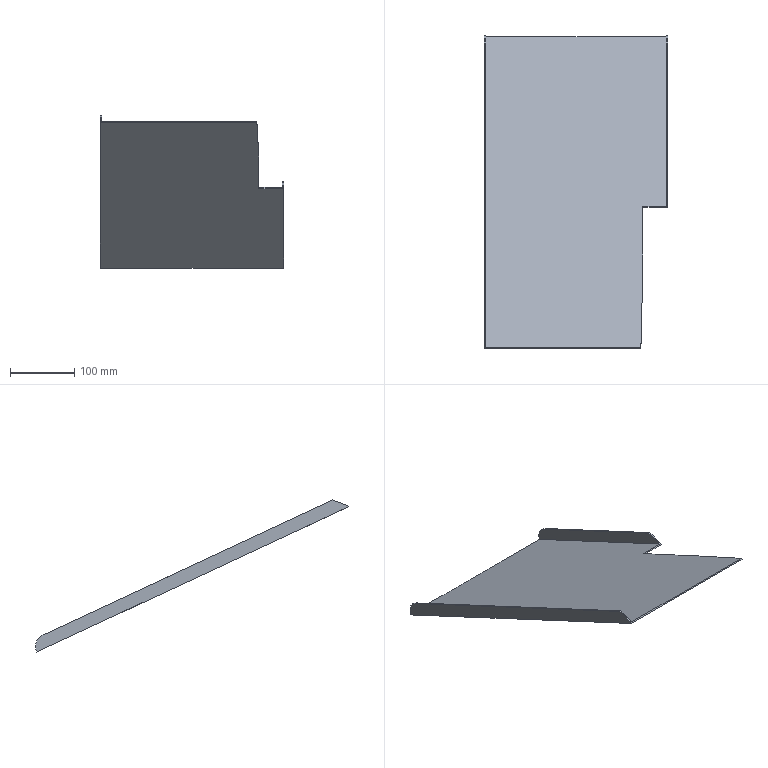Part | NX | features solid 2 | 1 solid | 17 faces | box 284.627 x 485.226 x 235.91 mm | volume 312843 mm3 | plane 14 | cylinder 2 | spline 1 | commonest cylinder face diameters 40 x2
STEP:
#1=CARTESIAN_POINT('',(-367.373,820.,-334.717));
#2=VERTEX_POINT('',#1);
#3=CARTESIAN_POINT('',(-367.373,820.,-332.51));
#4=VERTEX_POINT('',#3);
#5=CARTESIAN_POINT('',(-367.373,820.,-700.));
#6=DIRECTION('',(0.,0.,1.));
#7=VECTOR('',#6,1000.);
#8=LINE('',#5,#7);
#9=EDGE_CURVE('',#2,#4,#8,.T.);
#10=ORIENTED_EDGE('',*,*,#9,.F.);
#11=CARTESIAN_POINT('',(-648.,820.,-334.717));
#12=VERTEX_POINT('',#11);
#13=CARTESIAN_POINT('',(-419.852,820.,-334.717));
#14=DIRECTION('',(-1.,0.,0.));
#15=VECTOR('',#14,1000.);
#16=LINE('',#13,#15);
#17=EDGE_CURVE('',#2,#12,#16,.T.);
#18=ORIENTED_EDGE('',*,*,#17,.T.);
#19=CARTESIAN_POINT('',(-648.,820.,-332.51));
#20=VERTEX_POINT('',#19);
#21=CARTESIAN_POINT('',(-648.,820.,-700.));
#22=DIRECTION('',(0.,0.,-1.));
#23=VECTOR('',#22,1000.);
#24=LINE('',#21,#23);
#25=EDGE_CURVE('',#20,#12,#24,.T.);
#26=ORIENTED_EDGE('',*,*,#25,.F.);
#27=CARTESIAN_POINT('',(-419.852,820.,-332.51));
#28=DIRECTION('',(-1.,0.,0.));
#29=VECTOR('',#28,1000.);
#30=LINE('',#27,#29);
#31=EDGE_CURVE('',#4,#20,#30,.T.);
#32=ORIENTED_EDGE('',*,*,#31,.F.);
#33=EDGE_LOOP('',(#10,#18,#26,#32));
#34=FACE_BOUND('',#33,.T.);
#35=CARTESIAN_POINT('',(1065.,820.,-700.));
#36=DIRECTION('',(0.,-1.,0.));
#37=DIRECTION('',(-1.,0.,0.));
#38=AXIS2_PLACEMENT_3D('',#35,#36,#37);
#39=PLANE('',#38);
#40=ADVANCED_FACE('',(#34),#39,.F.);
#41=CARTESIAN_POINT('',(-367.373,556.481,-209.629));
#42=VERTEX_POINT('',#41);
#43=CARTESIAN_POINT('',(-367.373,317.493,-98.187));
#44=DIRECTION('',(0.,-0.9063,0.4226));
#45=VECTOR('',#44,1000.);
#46=LINE('',#43,#45);
#47=EDGE_CURVE('',#4,#42,#46,.T.);
#48=ORIENTED_EDGE('',*,*,#47,.F.);
#49=ORIENTED_EDGE('',*,*,#31,.T.);
#50=CARTESIAN_POINT('',(-648.,337.493,-107.514));
#51=VERTEX_POINT('',#50);
#52=CARTESIAN_POINT('',(-648.,317.493,-98.187));
#53=DIRECTION('',(0.,0.9063,-0.4226));
#54=VECTOR('',#53,1000.);
#55=LINE('',#52,#54);
#56=EDGE_CURVE('',#51,#20,#55,.T.);
#57=ORIENTED_EDGE('',*,*,#56,.F.);
#58=CARTESIAN_POINT('',(-407.057,337.493,-107.514));
#59=VERTEX_POINT('',#58);
#60=CARTESIAN_POINT('',(-419.852,337.493,-107.514));
#61=DIRECTION('',(-1.,0.,0.));
#62=VECTOR('',#61,1000.);
#63=LINE('',#60,#62);
#64=EDGE_CURVE('',#51,#59,#63,.F.);
#65=ORIENTED_EDGE('',*,*,#64,.T.);
#66=CARTESIAN_POINT('',(-404.001,556.494,-209.635));
#67=VERTEX_POINT('',#66);
#68=CARTESIAN_POINT('',(-407.057,337.493,-107.514));
#69=CARTESIAN_POINT('',(-406.902,341.01,-109.153));
#70=CARTESIAN_POINT('',(-406.6,348.566,-112.677));
#71=CARTESIAN_POINT('',(-406.245,359.315,-117.689));
#72=CARTESIAN_POINT('',(-405.973,368.697,-122.064));
#73=CARTESIAN_POINT('',(-405.808,374.888,-124.951));
#74=CARTESIAN_POINT('',(-405.68,380.035,-127.351));
#75=CARTESIAN_POINT('',(-405.585,383.996,-129.198));
#76=CARTESIAN_POINT('',(-405.507,387.368,-130.77));
#77=CARTESIAN_POINT('',(-405.453,389.792,-131.901));
#78=CARTESIAN_POINT('',(-405.423,391.156,-132.537));
#79=CARTESIAN_POINT('',(-405.399,392.28,-133.061));
#80=CARTESIAN_POINT('',(-405.382,393.048,-133.419));
#81=CARTESIAN_POINT('',(-405.358,394.196,-133.954));
#82=CARTESIAN_POINT('',(-405.316,396.148,-134.865));
#83=CARTESIAN_POINT('',(-405.258,398.972,-136.182));
#84=CARTESIAN_POINT('',(-405.19,402.355,-137.759));
#85=CARTESIAN_POINT('',(-405.102,406.878,-139.868));
#86=CARTESIAN_POINT('',(-404.997,412.548,-142.512));
#87=CARTESIAN_POINT('',(-404.84,421.657,-146.76));
#88=CARTESIAN_POINT('',(-404.699,430.812,-151.029));
#89=CARTESIAN_POINT('',(-404.589,438.887,-154.794));
#90=CARTESIAN_POINT('',(-404.531,443.489,-156.94));
#91=CARTESIAN_POINT('',(-404.488,447.022,-158.587));
#92=CARTESIAN_POINT('',(-404.45,450.273,-160.103));
#93=CARTESIAN_POINT('',(-404.401,454.73,-162.182));
#94=CARTESIAN_POINT('',(-404.322,462.533,-165.821));
#95=CARTESIAN_POINT('',(-404.245,471.588,-170.043));
#96=CARTESIAN_POINT('',(-404.181,480.752,-174.316));
#97=CARTESIAN_POINT('',(-404.147,486.53,-177.01));
#98=CARTESIAN_POINT('',(-404.123,491.18,-179.179));
#99=CARTESIAN_POINT('',(-404.107,494.685,-180.813));
#100=CARTESIAN_POINT('',(-404.095,497.607,-182.176));
#101=CARTESIAN_POINT('',(-404.087,499.681,-183.143));
#102=CARTESIAN_POINT('',(-404.083,500.833,-183.68));
#103=CARTESIAN_POINT('',(-404.079,501.795,-184.129));
#104=CARTESIAN_POINT('',(-404.078,502.388,-184.405));
#105=CARTESIAN_POINT('',(-404.074,503.324,-184.842));
#106=CARTESIAN_POINT('',(-404.069,504.937,-185.594));
#107=CARTESIAN_POINT('',(-404.063,507.377,-186.732));
#108=CARTESIAN_POINT('',(-404.055,510.455,-188.167));
#109=CARTESIAN_POINT('',(-404.046,514.785,-190.186));
#110=CARTESIAN_POINT('',(-404.037,519.44,-192.357));
#111=CARTESIAN_POINT('',(-404.031,524.43,-194.684));
#112=CARTESIAN_POINT('',(-404.027,527.677,-196.198));
#113=CARTESIAN_POINT('',(-404.024,530.378,-197.457));
#114=CARTESIAN_POINT('',(-404.022,531.884,-198.159));
#115=CARTESIAN_POINT('',(-404.021,532.972,-198.667));
#116=CARTESIAN_POINT('',(-404.021,533.53,-198.927));
#117=CARTESIAN_POINT('',(-404.02,534.536,-199.396));
#118=CARTESIAN_POINT('',(-404.018,536.527,-200.325));
#119=CARTESIAN_POINT('',(-404.016,539.382,-201.656));
#120=CARTESIAN_POINT('',(-404.012,543.944,-203.783));
#121=CARTESIAN_POINT('',(-404.007,549.649,-206.444));
#122=CARTESIAN_POINT('',(-404.003,554.212,-208.571));
#123=CARTESIAN_POINT('',(-404.001,556.494,-209.635));
#124=B_SPLINE_CURVE_WITH_KNOTS('',3,(#68,#69,#70,#71,#72,#73,#74,#75,#76,#77,#78,#79,#80,#81,#82,#83,#84,#85,#86,#87,#88,#89,#90,#91,#92,#93,#94,#95,#96,#97,#98,#99,#100,#101,#102,#103,#104,#105,#106,#107,#108,#109,#110,#111,#112,#113,#114,#115,#116,#117,#118,#119,#120,#121,#122,#123),.UNSPECIFIED.,.F.,.F.,(4,1,1,1,1,1,1,1,1,1,1,1,1,1,1,1,1,1,1,1,1,1,1,1,1,1,1,1,1,1,1,1,1,1,1,1,1,1,1,1,1,1,1,1,1,1,1,1,1,1,1,1,1,4),(0.,0.0625,0.125,0.1562,0.1875,0.2031,0.2188,0.2344,0.2422,0.2461,0.25,0.2539,0.2578,0.2656,0.2812,0.2969,0.3125,0.3438,0.375,0.4375,0.4688,0.4844,0.5,0.5156,0.5312,0.5625,0.625,0.6562,0.6875,0.7031,0.7188,0.7344,0.7422,0.7461,0.75,0.7539,0.7578,0.7656,0.7812,0.7969,0.8125,0.8438,0.8594,0.875,0.8828,0.8906,0.8926,0.8945,0.8984,0.9062,0.9219,0.9375,0.9688,1.),.UNSPECIFIED.);
#125=EDGE_CURVE('',#67,#59,#124,.F.);
#126=ORIENTED_EDGE('',*,*,#125,.F.);
#127=CARTESIAN_POINT('',(-404.001,556.494,-209.635));
#128=CARTESIAN_POINT('',(-391.792,556.49,-209.633));
#129=CARTESIAN_POINT('',(-379.582,556.485,-209.631));
#130=CARTESIAN_POINT('',(-367.373,556.481,-209.629));
#131=B_SPLINE_CURVE_WITH_KNOTS('',3,(#127,#128,#129,#130),.UNSPECIFIED.,.F.,.F.,(4,4),(0.,0.9482),.UNSPECIFIED.);
#132=EDGE_CURVE('',#67,#42,#131,.T.);
#133=ORIENTED_EDGE('',*,*,#132,.T.);
#134=EDGE_LOOP('',(#48,#49,#57,#65,#126,#133));
#135=FACE_BOUND('',#134,.T.);
#136=CARTESIAN_POINT('',(-419.852,317.493,-98.187));
#137=DIRECTION('',(0.,-0.4226,-0.9063));
#138=DIRECTION('',(-1.,0.,0.));
#139=AXIS2_PLACEMENT_3D('',#136,#137,#138);
#140=PLANE('',#139);
#141=ADVANCED_FACE('',(#135),#140,.F.);
#142=CARTESIAN_POINT('',(-367.373,555.635,-211.442));
#143=VERTEX_POINT('',#142);
#144=CARTESIAN_POINT('',(-367.373,556.481,-209.629));
#145=CARTESIAN_POINT('',(-367.373,556.199,-210.234));
#146=CARTESIAN_POINT('',(-367.373,555.917,-210.838));
#147=CARTESIAN_POINT('',(-367.373,555.635,-211.443));
#148=B_SPLINE_CURVE_WITH_KNOTS('',3,(#144,#145,#146,#147),.UNSPECIFIED.,.F.,.F.,(4,4),(0.,1.),.UNSPECIFIED.);
#149=EDGE_CURVE('',#143,#42,#148,.F.);
#150=ORIENTED_EDGE('',*,*,#149,.T.);
#151=ORIENTED_EDGE('',*,*,#132,.F.);
#152=CARTESIAN_POINT('',(-404.001,555.649,-211.448));
#153=VERTEX_POINT('',#152);
#154=CARTESIAN_POINT('',(-404.001,556.494,-209.635));
#155=CARTESIAN_POINT('',(-404.001,556.212,-210.24));
#156=CARTESIAN_POINT('',(-404.001,555.931,-210.844));
#157=CARTESIAN_POINT('',(-404.001,555.649,-211.448));
#158=B_SPLINE_CURVE_WITH_KNOTS('',3,(#154,#155,#156,#157),.UNSPECIFIED.,.F.,.F.,(4,4),(0.,1.),.UNSPECIFIED.);
#159=EDGE_CURVE('',#67,#153,#158,.T.);
#160=ORIENTED_EDGE('',*,*,#159,.T.);
#161=CARTESIAN_POINT('',(-404.001,555.649,-211.448));
#162=CARTESIAN_POINT('',(-391.792,555.644,-211.446));
#163=CARTESIAN_POINT('',(-379.582,555.64,-211.444));
#164=CARTESIAN_POINT('',(-367.373,555.635,-211.442));
#165=B_SPLINE_CURVE_WITH_KNOTS('',3,(#161,#162,#163,#164),.UNSPECIFIED.,.F.,.F.,(4,4),(0.,0.9482),.UNSPECIFIED.);
#166=EDGE_CURVE('',#153,#143,#165,.T.);
#167=ORIENTED_EDGE('',*,*,#166,.T.);
#168=EDGE_LOOP('',(#150,#151,#160,#167));
#169=FACE_BOUND('',#168,.T.);
#170=CARTESIAN_POINT('',(-404.001,556.494,-209.635));
#171=DIRECTION('',(0.0004088,0.9063,-0.4226));
#172=DIRECTION('',(0.,0.4226,0.9063));
#173=AXIS2_PLACEMENT_3D('',#170,#171,#172);
#174=PLANE('',#173);
#175=ADVANCED_FACE('',(#169),#174,.F.);
#176=CARTESIAN_POINT('',(-365.373,555.635,-211.441));
#177=VERTEX_POINT('',#176);
#178=CARTESIAN_POINT('',(-365.373,820.,-334.717));
#179=VERTEX_POINT('',#178);
#180=CARTESIAN_POINT('',(-365.373,543.591,-205.825));
#181=DIRECTION('',(0.,-0.9063,0.4226));
#182=VECTOR('',#181,1000.);
#183=LINE('',#180,#182);
#184=EDGE_CURVE('',#177,#179,#183,.F.);
#185=ORIENTED_EDGE('',*,*,#184,.T.);
#186=CARTESIAN_POINT('',(-365.373,810.326,-308.138));
#187=VERTEX_POINT('',#186);
#188=CARTESIAN_POINT('',(-365.373,801.874,-326.265));
#189=DIRECTION('',(1.,0.,0.));
#190=DIRECTION('',(0.,1.,0.));
#191=AXIS2_PLACEMENT_3D('',#188,#189,#190);
#192=CIRCLE('',#191,20.);
#193=EDGE_CURVE('',#179,#187,#192,.T.);
#194=ORIENTED_EDGE('',*,*,#193,.T.);
#195=CARTESIAN_POINT('',(-365.373,580.401,-200.922));
#196=VERTEX_POINT('',#195);
#197=CARTESIAN_POINT('',(-365.373,564.087,-193.315));
#198=DIRECTION('',(0.,0.9063,-0.4226));
#199=VECTOR('',#198,1000.);
#200=LINE('',#197,#199);
#201=EDGE_CURVE('',#196,#187,#200,.T.);
#202=ORIENTED_EDGE('',*,*,#201,.F.);
#203=CARTESIAN_POINT('',(-365.373,556.48,-209.629));
#204=VERTEX_POINT('',#203);
#205=CARTESIAN_POINT('',(-365.373,555.151,-210.112));
#206=DIRECTION('',(0.,0.9397,0.342));
#207=VECTOR('',#206,1000.);
#208=LINE('',#205,#207);
#209=EDGE_CURVE('',#196,#204,#208,.F.);
#210=ORIENTED_EDGE('',*,*,#209,.T.);
#211=CARTESIAN_POINT('',(-365.373,556.48,-209.629));
#212=CARTESIAN_POINT('',(-365.373,556.198,-210.233));
#213=CARTESIAN_POINT('',(-365.373,555.916,-210.837));
#214=CARTESIAN_POINT('',(-365.373,555.635,-211.441));
#215=B_SPLINE_CURVE_WITH_KNOTS('',3,(#211,#212,#213,#214),.UNSPECIFIED.,.F.,.F.,(4,4),(0.,1.),.UNSPECIFIED.);
#216=EDGE_CURVE('',#177,#204,#215,.F.);
#217=ORIENTED_EDGE('',*,*,#216,.F.);
#218=EDGE_LOOP('',(#185,#194,#202,#210,#217));
#219=FACE_BOUND('',#218,.T.);
#220=CARTESIAN_POINT('',(-365.373,544.437,-204.013));
#221=DIRECTION('',(-1.,0.,0.));
#222=DIRECTION('',(0.,-1.,0.));
#223=AXIS2_PLACEMENT_3D('',#220,#221,#222);
#224=PLANE('',#223);
#225=ADVANCED_FACE('',(#219),#224,.F.);
#226=CARTESIAN_POINT('',(-650.,810.326,-308.138));
#227=VERTEX_POINT('',#226);
#228=CARTESIAN_POINT('',(-650.,820.,-334.717));
#229=VERTEX_POINT('',#228);
#230=CARTESIAN_POINT('',(-650.,801.874,-326.265));
#231=DIRECTION('',(-1.,0.,0.));
#232=DIRECTION('',(0.,0.,1.));
#233=AXIS2_PLACEMENT_3D('',#230,#231,#232);
#234=CIRCLE('',#233,20.);
#235=EDGE_CURVE('',#227,#229,#234,.T.);
#236=ORIENTED_EDGE('',*,*,#235,.T.);
#237=CARTESIAN_POINT('',(-650.,336.648,-109.326));
#238=VERTEX_POINT('',#237);
#239=CARTESIAN_POINT('',(-650.,-1117.742,568.867));
#240=DIRECTION('',(0.,-0.9063,0.4226));
#241=VECTOR('',#240,1000.);
#242=LINE('',#239,#241);
#243=EDGE_CURVE('',#229,#238,#242,.T.);
#244=ORIENTED_EDGE('',*,*,#243,.T.);
#245=CARTESIAN_POINT('',(-650.,337.493,-107.514));
#246=VERTEX_POINT('',#245);
#247=CARTESIAN_POINT('',(-650.,337.493,-107.514));
#248=DIRECTION('',(0.,-0.4226,-0.9063));
#249=VECTOR('',#248,1000.);
#250=LINE('',#247,#249);
#251=EDGE_CURVE('',#246,#238,#250,.T.);
#252=ORIENTED_EDGE('',*,*,#251,.F.);
#253=CARTESIAN_POINT('',(-650.,361.414,-98.807));
#254=VERTEX_POINT('',#253);
#255=CARTESIAN_POINT('',(-650.,690.536,20.983));
#256=DIRECTION('',(0.,0.9397,0.342));
#257=VECTOR('',#256,1000.);
#258=LINE('',#255,#257);
#259=EDGE_CURVE('',#246,#254,#258,.T.);
#260=ORIENTED_EDGE('',*,*,#259,.T.);
#261=CARTESIAN_POINT('',(-650.,828.452,-316.591));
#262=DIRECTION('',(0.,-0.9063,0.4226));
#263=VECTOR('',#262,1000.);
#264=LINE('',#261,#263);
#265=EDGE_CURVE('',#227,#254,#264,.T.);
#266=ORIENTED_EDGE('',*,*,#265,.F.);
#267=EDGE_LOOP('',(#236,#244,#252,#260,#266));
#268=FACE_BOUND('',#267,.T.);
#269=CARTESIAN_POINT('',(-650.,-1116.896,570.679));
#270=DIRECTION('',(1.,0.,0.));
#271=DIRECTION('',(0.,0.,-1.));
#272=AXIS2_PLACEMENT_3D('',#269,#270,#271);
#273=PLANE('',#272);
#274=ADVANCED_FACE('',(#268),#273,.F.);
#275=CARTESIAN_POINT('',(-407.057,336.648,-109.326));
#276=VERTEX_POINT('',#275);
#277=CARTESIAN_POINT('',(-419.852,336.648,-109.326));
#278=DIRECTION('',(-1.,0.,0.));
#279=VECTOR('',#278,1000.);
#280=LINE('',#277,#279);
#281=EDGE_CURVE('',#238,#276,#280,.F.);
#282=ORIENTED_EDGE('',*,*,#281,.T.);
#283=CARTESIAN_POINT('',(-407.057,336.648,-109.326));
#284=CARTESIAN_POINT('',(-407.057,336.93,-108.722));
#285=CARTESIAN_POINT('',(-407.057,337.212,-108.118));
#286=CARTESIAN_POINT('',(-407.057,337.493,-107.514));
#287=B_SPLINE_CURVE_WITH_KNOTS('',3,(#283,#284,#285,#286),.UNSPECIFIED.,.F.,.F.,(4,4),(0.,1.),.UNSPECIFIED.);
#288=EDGE_CURVE('',#59,#276,#287,.F.);
#289=ORIENTED_EDGE('',*,*,#288,.F.);
#290=ORIENTED_EDGE('',*,*,#64,.F.);
#291=CARTESIAN_POINT('',(-419.852,337.493,-107.514));
#292=DIRECTION('',(-1.,0.,0.));
#293=VECTOR('',#292,1000.);
#294=LINE('',#291,#293);
#295=EDGE_CURVE('',#246,#51,#294,.F.);
#296=ORIENTED_EDGE('',*,*,#295,.F.);
#297=ORIENTED_EDGE('',*,*,#251,.T.);
#298=EDGE_LOOP('',(#282,#289,#290,#296,#297));
#299=FACE_BOUND('',#298,.T.);
#300=CARTESIAN_POINT('',(-419.852,337.493,-107.514));
#301=DIRECTION('',(0.,0.9063,-0.4226));
#302=DIRECTION('',(0.,0.4226,0.9063));
#303=AXIS2_PLACEMENT_3D('',#300,#301,#302);
#304=PLANE('',#303);
#305=ADVANCED_FACE('',(#299),#304,.F.);
#306=CARTESIAN_POINT('',(-407.057,336.648,-109.326));
#307=CARTESIAN_POINT('',(-406.902,340.165,-110.966));
#308=CARTESIAN_POINT('',(-406.6,347.721,-114.489));
#309=CARTESIAN_POINT('',(-406.245,358.47,-119.502));
#310=CARTESIAN_POINT('',(-405.973,367.852,-123.877));
#311=CARTESIAN_POINT('',(-405.808,374.042,-126.763));
#312=CARTESIAN_POINT('',(-405.68,379.189,-129.163));
#313=CARTESIAN_POINT('',(-405.585,383.151,-131.011));
#314=CARTESIAN_POINT('',(-405.507,386.522,-132.583));
#315=CARTESIAN_POINT('',(-405.453,388.947,-133.714));
#316=CARTESIAN_POINT('',(-405.423,390.311,-134.35));
#317=CARTESIAN_POINT('',(-405.399,391.435,-134.874));
#318=CARTESIAN_POINT('',(-405.382,392.202,-135.232));
#319=CARTESIAN_POINT('',(-405.358,393.351,-135.767));
#320=CARTESIAN_POINT('',(-405.316,395.303,-136.677));
#321=CARTESIAN_POINT('',(-405.258,398.127,-137.994));
#322=CARTESIAN_POINT('',(-405.19,401.51,-139.572));
#323=CARTESIAN_POINT('',(-405.102,406.033,-141.681));
#324=CARTESIAN_POINT('',(-404.997,411.703,-144.325));
#325=CARTESIAN_POINT('',(-404.84,420.811,-148.572));
#326=CARTESIAN_POINT('',(-404.699,429.967,-152.841));
#327=CARTESIAN_POINT('',(-404.589,438.042,-156.607));
#328=CARTESIAN_POINT('',(-404.531,442.643,-158.753));
#329=CARTESIAN_POINT('',(-404.488,446.176,-160.4));
#330=CARTESIAN_POINT('',(-404.45,449.427,-161.916));
#331=CARTESIAN_POINT('',(-404.401,453.885,-163.995));
#332=CARTESIAN_POINT('',(-404.322,461.688,-167.633));
#333=CARTESIAN_POINT('',(-404.245,470.743,-171.856));
#334=CARTESIAN_POINT('',(-404.181,479.907,-176.129));
#335=CARTESIAN_POINT('',(-404.147,485.685,-178.823));
#336=CARTESIAN_POINT('',(-404.123,490.334,-180.991));
#337=CARTESIAN_POINT('',(-404.107,493.84,-182.626));
#338=CARTESIAN_POINT('',(-404.095,496.762,-183.988));
#339=CARTESIAN_POINT('',(-404.087,498.835,-184.955));
#340=CARTESIAN_POINT('',(-404.083,499.988,-185.493));
#341=CARTESIAN_POINT('',(-404.079,500.95,-185.941));
#342=CARTESIAN_POINT('',(-404.078,501.543,-186.218));
#343=CARTESIAN_POINT('',(-404.074,502.479,-186.654));
#344=CARTESIAN_POINT('',(-404.069,504.092,-187.407));
#345=CARTESIAN_POINT('',(-404.063,506.532,-188.544));
#346=CARTESIAN_POINT('',(-404.055,509.61,-189.98));
#347=CARTESIAN_POINT('',(-404.046,513.939,-191.998));
#348=CARTESIAN_POINT('',(-404.037,518.595,-194.169));
#349=CARTESIAN_POINT('',(-404.031,523.585,-196.496));
#350=CARTESIAN_POINT('',(-404.027,526.832,-198.01));
#351=CARTESIAN_POINT('',(-404.024,529.533,-199.27));
#352=CARTESIAN_POINT('',(-404.022,531.039,-199.972));
#353=CARTESIAN_POINT('',(-404.021,532.126,-200.479));
#354=CARTESIAN_POINT('',(-404.021,532.685,-200.74));
#355=CARTESIAN_POINT('',(-404.02,533.691,-201.209));
#356=CARTESIAN_POINT('',(-404.018,535.682,-202.137));
#357=CARTESIAN_POINT('',(-404.016,538.537,-203.469));
#358=CARTESIAN_POINT('',(-404.012,543.099,-205.596));
#359=CARTESIAN_POINT('',(-404.007,548.804,-208.256));
#360=CARTESIAN_POINT('',(-404.003,553.367,-210.384));
#361=CARTESIAN_POINT('',(-404.001,555.649,-211.448));
#362=B_SPLINE_CURVE_WITH_KNOTS('',3,(#306,#307,#308,#309,#310,#311,#312,#313,#314,#315,#316,#317,#318,#319,#320,#321,#322,#323,#324,#325,#326,#327,#328,#329,#330,#331,#332,#333,#334,#335,#336,#337,#338,#339,#340,#341,#342,#343,#344,#345,#346,#347,#348,#349,#350,#351,#352,#353,#354,#355,#356,#357,#358,#359,#360,#361),.UNSPECIFIED.,.F.,.F.,(4,1,1,1,1,1,1,1,1,1,1,1,1,1,1,1,1,1,1,1,1,1,1,1,1,1,1,1,1,1,1,1,1,1,1,1,1,1,1,1,1,1,1,1,1,1,1,1,1,1,1,1,1,4),(0.,0.0625,0.125,0.1562,0.1875,0.2031,0.2188,0.2344,0.2422,0.2461,0.25,0.2539,0.2578,0.2656,0.2812,0.2969,0.3125,0.3438,0.375,0.4375,0.4688,0.4844,0.5,0.5156,0.5312,0.5625,0.625,0.6562,0.6875,0.7031,0.7188,0.7344,0.7422,0.7461,0.75,0.7539,0.7578,0.7656,0.7812,0.7969,0.8125,0.8438,0.8594,0.875,0.8828,0.8906,0.8926,0.8945,0.8984,0.9062,0.9219,0.9375,0.9688,1.),.UNSPECIFIED.);
#363=EDGE_CURVE('',#153,#276,#362,.F.);
#364=ORIENTED_EDGE('',*,*,#363,.F.);
#365=ORIENTED_EDGE('',*,*,#159,.F.);
#366=ORIENTED_EDGE('',*,*,#125,.T.);
#367=ORIENTED_EDGE('',*,*,#288,.T.);
#368=EDGE_LOOP('',(#364,#365,#366,#367));
#369=FACE_BOUND('',#368,.T.);
#370=CARTESIAN_POINT('',(-407.057,337.493,-107.514));
#371=CARTESIAN_POINT('',(-407.057,336.648,-109.326));
#372=CARTESIAN_POINT('',(-406.902,341.01,-109.153));
#373=CARTESIAN_POINT('',(-406.902,340.165,-110.966));
#374=CARTESIAN_POINT('',(-406.6,348.566,-112.677));
#375=CARTESIAN_POINT('',(-406.6,347.721,-114.489));
#376=CARTESIAN_POINT('',(-406.245,359.315,-117.689));
#377=CARTESIAN_POINT('',(-406.245,358.47,-119.502));
#378=CARTESIAN_POINT('',(-405.973,368.697,-122.064));
#379=CARTESIAN_POINT('',(-405.973,367.852,-123.877));
#380=CARTESIAN_POINT('',(-405.808,374.888,-124.951));
#381=CARTESIAN_POINT('',(-405.808,374.042,-126.763));
#382=CARTESIAN_POINT('',(-405.68,380.035,-127.351));
#383=CARTESIAN_POINT('',(-405.68,379.189,-129.163));
#384=CARTESIAN_POINT('',(-405.585,383.996,-129.198));
#385=CARTESIAN_POINT('',(-405.585,383.151,-131.011));
#386=CARTESIAN_POINT('',(-405.507,387.368,-130.77));
#387=CARTESIAN_POINT('',(-405.507,386.522,-132.583));
#388=CARTESIAN_POINT('',(-405.453,389.792,-131.901));
#389=CARTESIAN_POINT('',(-405.453,388.947,-133.714));
#390=CARTESIAN_POINT('',(-405.423,391.156,-132.537));
#391=CARTESIAN_POINT('',(-405.423,390.311,-134.35));
#392=CARTESIAN_POINT('',(-405.399,392.28,-133.061));
#393=CARTESIAN_POINT('',(-405.399,391.435,-134.874));
#394=CARTESIAN_POINT('',(-405.382,393.048,-133.419));
#395=CARTESIAN_POINT('',(-405.382,392.202,-135.232));
#396=CARTESIAN_POINT('',(-405.358,394.196,-133.954));
#397=CARTESIAN_POINT('',(-405.358,393.351,-135.767));
#398=CARTESIAN_POINT('',(-405.316,396.148,-134.865));
#399=CARTESIAN_POINT('',(-405.316,395.303,-136.677));
#400=CARTESIAN_POINT('',(-405.258,398.972,-136.182));
#401=CARTESIAN_POINT('',(-405.258,398.127,-137.994));
#402=CARTESIAN_POINT('',(-405.19,402.355,-137.759));
#403=CARTESIAN_POINT('',(-405.19,401.51,-139.572));
#404=CARTESIAN_POINT('',(-405.102,406.878,-139.868));
#405=CARTESIAN_POINT('',(-405.102,406.033,-141.681));
#406=CARTESIAN_POINT('',(-404.997,412.548,-142.512));
#407=CARTESIAN_POINT('',(-404.997,411.703,-144.325));
#408=CARTESIAN_POINT('',(-404.84,421.657,-146.76));
#409=CARTESIAN_POINT('',(-404.84,420.811,-148.572));
#410=CARTESIAN_POINT('',(-404.699,430.812,-151.029));
#411=CARTESIAN_POINT('',(-404.699,429.967,-152.841));
#412=CARTESIAN_POINT('',(-404.589,438.887,-154.794));
#413=CARTESIAN_POINT('',(-404.589,438.042,-156.607));
#414=CARTESIAN_POINT('',(-404.531,443.489,-156.94));
#415=CARTESIAN_POINT('',(-404.531,442.643,-158.753));
#416=CARTESIAN_POINT('',(-404.488,447.022,-158.587));
#417=CARTESIAN_POINT('',(-404.488,446.176,-160.4));
#418=CARTESIAN_POINT('',(-404.45,450.273,-160.103));
#419=CARTESIAN_POINT('',(-404.45,449.427,-161.916));
#420=CARTESIAN_POINT('',(-404.401,454.73,-162.182));
#421=CARTESIAN_POINT('',(-404.401,453.885,-163.995));
#422=CARTESIAN_POINT('',(-404.322,462.533,-165.821));
#423=CARTESIAN_POINT('',(-404.322,461.688,-167.633));
#424=CARTESIAN_POINT('',(-404.245,471.588,-170.043));
#425=CARTESIAN_POINT('',(-404.245,470.743,-171.856));
#426=CARTESIAN_POINT('',(-404.181,480.752,-174.316));
#427=CARTESIAN_POINT('',(-404.181,479.907,-176.129));
#428=CARTESIAN_POINT('',(-404.147,486.53,-177.01));
#429=CARTESIAN_POINT('',(-404.147,485.685,-178.823));
#430=CARTESIAN_POINT('',(-404.123,491.18,-179.179));
#431=CARTESIAN_POINT('',(-404.123,490.334,-180.991));
#432=CARTESIAN_POINT('',(-404.107,494.685,-180.813));
#433=CARTESIAN_POINT('',(-404.107,493.84,-182.626));
#434=CARTESIAN_POINT('',(-404.095,497.607,-182.176));
#435=CARTESIAN_POINT('',(-404.095,496.762,-183.988));
#436=CARTESIAN_POINT('',(-404.087,499.681,-183.143));
#437=CARTESIAN_POINT('',(-404.087,498.835,-184.955));
#438=CARTESIAN_POINT('',(-404.083,500.833,-183.68));
#439=CARTESIAN_POINT('',(-404.083,499.988,-185.493));
#440=CARTESIAN_POINT('',(-404.079,501.795,-184.129));
#441=CARTESIAN_POINT('',(-404.079,500.95,-185.941));
#442=CARTESIAN_POINT('',(-404.078,502.388,-184.405));
#443=CARTESIAN_POINT('',(-404.078,501.543,-186.218));
#444=CARTESIAN_POINT('',(-404.074,503.324,-184.842));
#445=CARTESIAN_POINT('',(-404.074,502.479,-186.654));
#446=CARTESIAN_POINT('',(-404.069,504.937,-185.594));
#447=CARTESIAN_POINT('',(-404.069,504.092,-187.407));
#448=CARTESIAN_POINT('',(-404.063,507.377,-186.732));
#449=CARTESIAN_POINT('',(-404.063,506.532,-188.544));
#450=CARTESIAN_POINT('',(-404.055,510.455,-188.167));
#451=CARTESIAN_POINT('',(-404.055,509.61,-189.98));
#452=CARTESIAN_POINT('',(-404.046,514.785,-190.186));
#453=CARTESIAN_POINT('',(-404.046,513.939,-191.998));
#454=CARTESIAN_POINT('',(-404.037,519.44,-192.357));
#455=CARTESIAN_POINT('',(-404.037,518.595,-194.169));
#456=CARTESIAN_POINT('',(-404.031,524.43,-194.684));
#457=CARTESIAN_POINT('',(-404.031,523.585,-196.496));
#458=CARTESIAN_POINT('',(-404.027,527.677,-196.198));
#459=CARTESIAN_POINT('',(-404.027,526.832,-198.01));
#460=CARTESIAN_POINT('',(-404.024,530.378,-197.457));
#461=CARTESIAN_POINT('',(-404.024,529.533,-199.27));
#462=CARTESIAN_POINT('',(-404.022,531.884,-198.159));
#463=CARTESIAN_POINT('',(-404.022,531.039,-199.972));
#464=CARTESIAN_POINT('',(-404.021,532.972,-198.667));
#465=CARTESIAN_POINT('',(-404.021,532.126,-200.479));
#466=CARTESIAN_POINT('',(-404.021,533.53,-198.927));
#467=CARTESIAN_POINT('',(-404.021,532.685,-200.74));
#468=CARTESIAN_POINT('',(-404.02,534.536,-199.396));
#469=CARTESIAN_POINT('',(-404.02,533.691,-201.209));
#470=CARTESIAN_POINT('',(-404.018,536.527,-200.325));
#471=CARTESIAN_POINT('',(-404.018,535.682,-202.137));
#472=CARTESIAN_POINT('',(-404.016,539.382,-201.656));
#473=CARTESIAN_POINT('',(-404.016,538.537,-203.469));
#474=CARTESIAN_POINT('',(-404.012,543.944,-203.783));
#475=CARTESIAN_POINT('',(-404.012,543.099,-205.596));
#476=CARTESIAN_POINT('',(-404.007,549.649,-206.444));
#477=CARTESIAN_POINT('',(-404.007,548.804,-208.256));
#478=CARTESIAN_POINT('',(-404.003,554.212,-208.571));
#479=CARTESIAN_POINT('',(-404.003,553.367,-210.384));
#480=CARTESIAN_POINT('',(-404.001,556.494,-209.635));
#481=CARTESIAN_POINT('',(-404.001,555.649,-211.448));
#482=B_SPLINE_SURFACE_WITH_KNOTS('',3,1,((#370,#371),(#372,#373),(#374,#375),(#376,#377),(#378,#379),(#380,#381),(#382,#383),(#384,#385),(#386,#387),(#388,#389),(#390,#391),(#392,#393),(#394,#395),(#396,#397),(#398,#399),(#400,#401),(#402,#403),(#404,#405),(#406,#407),(#408,#409),(#410,#411),(#412,#413),(#414,#415),(#416,#417),(#418,#419),(#420,#421),(#422,#423),(#424,#425),(#426,#427),(#428,#429),(#430,#431),(#432,#433),(#434,#435),(#436,#437),(#438,#439),(#440,#441),(#442,#443),(#444,#445),(#446,#447),(#448,#449),(#450,#451),(#452,#453),(#454,#455),(#456,#457),(#458,#459),(#460,#461),(#462,#463),(#464,#465),(#466,#467),(#468,#469),(#470,#471),(#472,#473),(#474,#475),(#476,#477),(#478,#479),(#480,#481)),.SURF_OF_LINEAR_EXTRUSION.,.F.,.F.,.F.,(4,1,1,1,1,1,1,1,1,1,1,1,1,1,1,1,1,1,1,1,1,1,1,1,1,1,1,1,1,1,1,1,1,1,1,1,1,1,1,1,1,1,1,1,1,1,1,1,1,1,1,1,1,4),(2,2),(0.,0.0625,0.125,0.1562,0.1875,0.2031,0.2188,0.2344,0.2422,0.2461,0.25,0.2539,0.2578,0.2656,0.2812,0.2969,0.3125,0.3438,0.375,0.4375,0.4688,0.4844,0.5,0.5156,0.5312,0.5625,0.625,0.6562,0.6875,0.7031,0.7188,0.7344,0.7422,0.7461,0.75,0.7539,0.7578,0.7656,0.7812,0.7969,0.8125,0.8438,0.8594,0.875,0.8828,0.8906,0.8926,0.8945,0.8984,0.9062,0.9219,0.9375,0.9688,1.),(0.,1.),.UNSPECIFIED.);
#483=ADVANCED_FACE('',(#369),#482,.F.);
#484=CARTESIAN_POINT('',(-367.373,555.635,-211.442));
#485=CARTESIAN_POINT('',(-366.706,555.635,-211.442));
#486=CARTESIAN_POINT('',(-366.039,555.635,-211.441));
#487=CARTESIAN_POINT('',(-365.373,555.635,-211.441));
#488=B_SPLINE_CURVE_WITH_KNOTS('',3,(#484,#485,#486,#487),.UNSPECIFIED.,.F.,.F.,(4,4),(0.9482,1.),.UNSPECIFIED.);
#489=EDGE_CURVE('',#177,#143,#488,.F.);
#490=ORIENTED_EDGE('',*,*,#489,.T.);
#491=ORIENTED_EDGE('',*,*,#166,.F.);
#492=ORIENTED_EDGE('',*,*,#363,.T.);
#493=ORIENTED_EDGE('',*,*,#281,.F.);
#494=ORIENTED_EDGE('',*,*,#243,.F.);
#495=CARTESIAN_POINT('',(-650.,820.,-334.717));
#496=DIRECTION('',(1.,0.,0.));
#497=VECTOR('',#496,1000.);
#498=LINE('',#495,#497);
#499=EDGE_CURVE('',#229,#12,#498,.T.);
#500=ORIENTED_EDGE('',*,*,#499,.T.);
#501=ORIENTED_EDGE('',*,*,#17,.F.);
#502=CARTESIAN_POINT('',(-419.852,820.,-334.717));
#503=DIRECTION('',(-1.,0.,0.));
#504=VECTOR('',#503,1000.);
#505=LINE('',#502,#504);
#506=EDGE_CURVE('',#179,#2,#505,.T.);
#507=ORIENTED_EDGE('',*,*,#506,.F.);
#508=ORIENTED_EDGE('',*,*,#184,.F.);
#509=EDGE_LOOP('',(#490,#491,#492,#493,#494,#500,#501,#507,#508));
#510=FACE_BOUND('',#509,.T.);
#511=CARTESIAN_POINT('',(-419.852,316.648,-100.));
#512=DIRECTION('',(0.,-0.4226,-0.9063));
#513=DIRECTION('',(-1.,0.,0.));
#514=AXIS2_PLACEMENT_3D('',#511,#512,#513);
#515=PLANE('',#514);
#516=ADVANCED_FACE('',(#510),#515,.T.);
#517=ORIENTED_EDGE('',*,*,#56,.T.);
#518=ORIENTED_EDGE('',*,*,#25,.T.);
#519=CARTESIAN_POINT('',(-648.,810.326,-308.138));
#520=VERTEX_POINT('',#519);
#521=CARTESIAN_POINT('',(-648.,801.874,-326.265));
#522=DIRECTION('',(-1.,0.,0.));
#523=DIRECTION('',(0.,0.,1.));
#524=AXIS2_PLACEMENT_3D('',#521,#522,#523);
#525=CIRCLE('',#524,20.);
#526=EDGE_CURVE('',#12,#520,#525,.F.);
#527=ORIENTED_EDGE('',*,*,#526,.T.);
#528=CARTESIAN_POINT('',(-648.,361.414,-98.807));
#529=VERTEX_POINT('',#528);
#530=CARTESIAN_POINT('',(-648.,828.452,-316.591));
#531=DIRECTION('',(0.,-0.9063,0.4226));
#532=VECTOR('',#531,1000.);
#533=LINE('',#530,#532);
#534=EDGE_CURVE('',#520,#529,#533,.T.);
#535=ORIENTED_EDGE('',*,*,#534,.T.);
#536=CARTESIAN_POINT('',(-648.,361.414,-98.807));
#537=DIRECTION('',(0.,-0.9397,-0.342));
#538=VECTOR('',#537,1000.);
#539=LINE('',#536,#538);
#540=EDGE_CURVE('',#529,#51,#539,.T.);
#541=ORIENTED_EDGE('',*,*,#540,.T.);
#542=EDGE_LOOP('',(#517,#518,#527,#535,#541));
#543=FACE_BOUND('',#542,.T.);
#544=CARTESIAN_POINT('',(-648.,820.,-334.717));
#545=DIRECTION('',(-1.,0.,0.));
#546=DIRECTION('',(0.,0.,1.));
#547=AXIS2_PLACEMENT_3D('',#544,#545,#546);
#548=PLANE('',#547);
#549=ADVANCED_FACE('',(#543),#548,.F.);
#550=ORIENTED_EDGE('',*,*,#265,.T.);
#551=CARTESIAN_POINT('',(-650.,361.414,-98.807));
#552=DIRECTION('',(-1.,0.,0.));
#553=VECTOR('',#552,1000.);
#554=LINE('',#551,#553);
#555=EDGE_CURVE('',#254,#529,#554,.F.);
#556=ORIENTED_EDGE('',*,*,#555,.T.);
#557=ORIENTED_EDGE('',*,*,#534,.F.);
#558=CARTESIAN_POINT('',(-650.,810.326,-308.138));
#559=DIRECTION('',(-1.,0.,0.));
#560=VECTOR('',#559,1000.);
#561=LINE('',#558,#560);
#562=EDGE_CURVE('',#520,#227,#561,.T.);
#563=ORIENTED_EDGE('',*,*,#562,.T.);
#564=EDGE_LOOP('',(#550,#556,#557,#563));
#565=FACE_BOUND('',#564,.T.);
#566=CARTESIAN_POINT('',(-650.,828.452,-316.591));
#567=DIRECTION('',(0.,-0.4226,-0.9063));
#568=DIRECTION('',(0.,-0.9063,0.4226));
#569=AXIS2_PLACEMENT_3D('',#566,#567,#568);
#570=PLANE('',#569);
#571=ADVANCED_FACE('',(#565),#570,.F.);
#572=ORIENTED_EDGE('',*,*,#235,.F.);
#573=ORIENTED_EDGE('',*,*,#562,.F.);
#574=ORIENTED_EDGE('',*,*,#526,.F.);
#575=ORIENTED_EDGE('',*,*,#499,.F.);
#576=EDGE_LOOP('',(#572,#573,#574,#575));
#577=FACE_BOUND('',#576,.T.);
#578=CARTESIAN_POINT('',(-650.,801.874,-326.265));
#579=DIRECTION('',(1.,0.,0.));
#580=DIRECTION('',(0.,0.,-1.));
#581=AXIS2_PLACEMENT_3D('',#578,#579,#580);
#582=CYLINDRICAL_SURFACE('',#581,20.);
#583=ADVANCED_FACE('',(#577),#582,.T.);
#584=ORIENTED_EDGE('',*,*,#259,.F.);
#585=ORIENTED_EDGE('',*,*,#295,.T.);
#586=ORIENTED_EDGE('',*,*,#540,.F.);
#587=ORIENTED_EDGE('',*,*,#555,.F.);
#588=EDGE_LOOP('',(#584,#585,#586,#587));
#589=FACE_BOUND('',#588,.T.);
#590=CARTESIAN_POINT('',(-650.,361.414,-98.807));
#591=DIRECTION('',(0.,-0.342,0.9397));
#592=DIRECTION('',(0.,-0.9397,-0.342));
#593=AXIS2_PLACEMENT_3D('',#590,#591,#592);
#594=PLANE('',#593);
#595=ADVANCED_FACE('',(#589),#594,.T.);
#596=CARTESIAN_POINT('',(-367.373,810.326,-308.138));
#597=VERTEX_POINT('',#596);
#598=CARTESIAN_POINT('',(-367.373,801.874,-326.265));
#599=DIRECTION('',(1.,0.,0.));
#600=DIRECTION('',(0.,1.,0.));
#601=AXIS2_PLACEMENT_3D('',#598,#599,#600);
#602=CIRCLE('',#601,20.);
#603=EDGE_CURVE('',#597,#2,#602,.F.);
#604=ORIENTED_EDGE('',*,*,#603,.T.);
#605=ORIENTED_EDGE('',*,*,#9,.T.);
#606=ORIENTED_EDGE('',*,*,#47,.T.);
#607=CARTESIAN_POINT('',(-367.373,580.401,-200.922));
#608=VERTEX_POINT('',#607);
#609=CARTESIAN_POINT('',(-367.373,556.48,-209.629));
#610=DIRECTION('',(0.,-0.9397,-0.342));
#611=VECTOR('',#610,1000.);
#612=LINE('',#609,#611);
#613=EDGE_CURVE('',#42,#608,#612,.F.);
#614=ORIENTED_EDGE('',*,*,#613,.T.);
#615=CARTESIAN_POINT('',(-367.373,564.087,-193.315));
#616=DIRECTION('',(0.,0.9063,-0.4226));
#617=VECTOR('',#616,1000.);
#618=LINE('',#615,#617);
#619=EDGE_CURVE('',#608,#597,#618,.T.);
#620=ORIENTED_EDGE('',*,*,#619,.T.);
#621=EDGE_LOOP('',(#604,#605,#606,#614,#620));
#622=FACE_BOUND('',#621,.T.);
#623=CARTESIAN_POINT('',(-367.373,555.635,-211.441));
#624=DIRECTION('',(1.,0.,0.));
#625=DIRECTION('',(0.,1.,0.));
#626=AXIS2_PLACEMENT_3D('',#623,#624,#625);
#627=PLANE('',#626);
#628=ADVANCED_FACE('',(#622),#627,.F.);
#629=ORIENTED_EDGE('',*,*,#619,.F.);
#630=CARTESIAN_POINT('',(-365.373,580.401,-200.922));
#631=DIRECTION('',(1.,0.,0.));
#632=VECTOR('',#631,1000.);
#633=LINE('',#630,#632);
#634=EDGE_CURVE('',#608,#196,#633,.T.);
#635=ORIENTED_EDGE('',*,*,#634,.T.);
#636=ORIENTED_EDGE('',*,*,#201,.T.);
#637=CARTESIAN_POINT('',(-365.373,810.326,-308.138));
#638=DIRECTION('',(1.,0.,0.));
#639=VECTOR('',#638,1000.);
#640=LINE('',#637,#639);
#641=EDGE_CURVE('',#187,#597,#640,.F.);
#642=ORIENTED_EDGE('',*,*,#641,.T.);
#643=EDGE_LOOP('',(#629,#635,#636,#642));
#644=FACE_BOUND('',#643,.T.);
#645=CARTESIAN_POINT('',(-365.373,564.087,-193.315));
#646=DIRECTION('',(0.,-0.4226,-0.9063));
#647=DIRECTION('',(0.,0.9063,-0.4226));
#648=AXIS2_PLACEMENT_3D('',#645,#646,#647);
#649=PLANE('',#648);
#650=ADVANCED_FACE('',(#644),#649,.F.);
#651=ORIENTED_EDGE('',*,*,#216,.T.);
#652=CARTESIAN_POINT('',(-365.373,556.48,-209.629));
#653=DIRECTION('',(-1.,0.,0.));
#654=VECTOR('',#653,1000.);
#655=LINE('',#652,#654);
#656=EDGE_CURVE('',#204,#42,#655,.T.);
#657=ORIENTED_EDGE('',*,*,#656,.T.);
#658=ORIENTED_EDGE('',*,*,#149,.F.);
#659=ORIENTED_EDGE('',*,*,#489,.F.);
#660=EDGE_LOOP('',(#651,#657,#658,#659));
#661=FACE_BOUND('',#660,.T.);
#662=CARTESIAN_POINT('',(-365.373,555.635,-211.441));
#663=DIRECTION('',(0.,0.9063,-0.4226));
#664=DIRECTION('',(0.,0.4226,0.9063));
#665=AXIS2_PLACEMENT_3D('',#662,#663,#664);
#666=PLANE('',#665);
#667=ADVANCED_FACE('',(#661),#666,.F.);
#668=ORIENTED_EDGE('',*,*,#193,.F.);
#669=ORIENTED_EDGE('',*,*,#506,.T.);
#670=ORIENTED_EDGE('',*,*,#603,.F.);
#671=ORIENTED_EDGE('',*,*,#641,.F.);
#672=EDGE_LOOP('',(#668,#669,#670,#671));
#673=FACE_BOUND('',#672,.T.);
#674=CARTESIAN_POINT('',(-365.373,801.874,-326.265));
#675=DIRECTION('',(1.,0.,0.));
#676=DIRECTION('',(0.,1.,0.));
#677=AXIS2_PLACEMENT_3D('',#674,#675,#676);
#678=CYLINDRICAL_SURFACE('',#677,20.);
#679=ADVANCED_FACE('',(#673),#678,.T.);
#680=ORIENTED_EDGE('',*,*,#209,.F.);
#681=ORIENTED_EDGE('',*,*,#634,.F.);
#682=ORIENTED_EDGE('',*,*,#613,.F.);
#683=ORIENTED_EDGE('',*,*,#656,.F.);
#684=EDGE_LOOP('',(#680,#681,#682,#683));
#685=FACE_BOUND('',#684,.T.);
#686=CARTESIAN_POINT('',(-365.373,556.48,-209.629));
#687=DIRECTION('',(0.,0.342,-0.9397));
#688=DIRECTION('',(0.,0.9397,0.342));
#689=AXIS2_PLACEMENT_3D('',#686,#687,#688);
#690=PLANE('',#689);
#691=ADVANCED_FACE('',(#685),#690,.F.);
#692=CLOSED_SHELL('',(#40,#141,#175,#225,#274,#305,#483,#516,#549,#571,#583,#595,#628,#650,#667,#679,#691));
#693=MANIFOLD_SOLID_BREP('',#692);
#694=(LENGTH_UNIT()NAMED_UNIT(*)SI_UNIT(.MILLI.,.METRE.));
#695=UNCERTAINTY_MEASURE_WITH_UNIT(LENGTH_MEASURE(0.0508),#694,'','');
#696=(NAMED_UNIT(*)PLANE_ANGLE_UNIT()SI_UNIT($,.RADIAN.));
#697=(NAMED_UNIT(*)SI_UNIT($,.STERADIAN.)SOLID_ANGLE_UNIT());
#698=(GEOMETRIC_REPRESENTATION_CONTEXT(3)GLOBAL_UNCERTAINTY_ASSIGNED_CONTEXT((#695))GLOBAL_UNIT_ASSIGNED_CONTEXT((#694,#696,#697))REPRESENTATION_CONTEXT('',''));
#699=ADVANCED_BREP_SHAPE_REPRESENTATION('',(#693),#698);